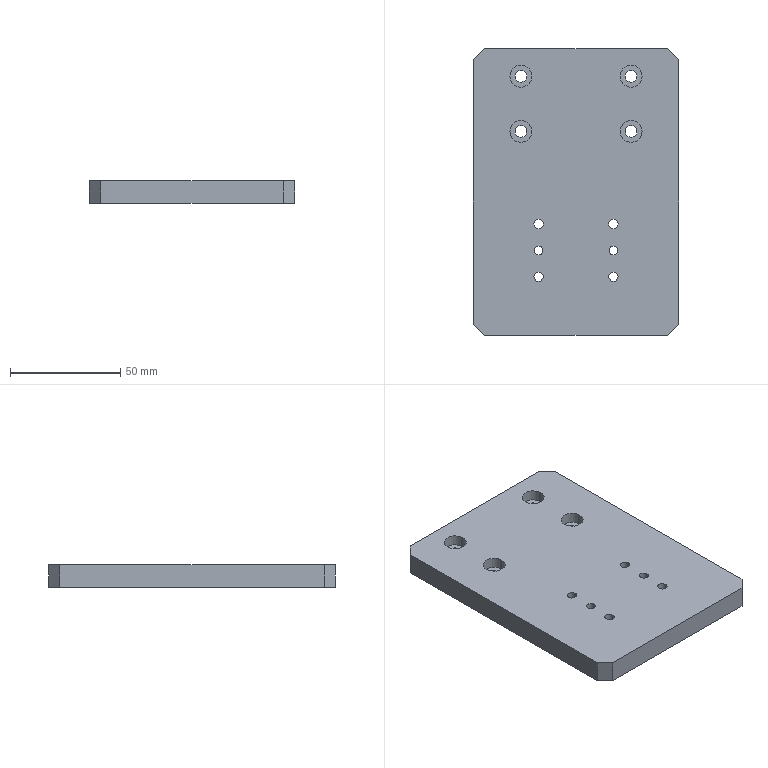Part | STEP file | CON-018 | 1 solid | 42 faces | box 93 x 130 x 10 mm | volume 117582 mm3 | cylinder 28 | plane 14 | commonest cylinder face diameters 4.2 x8 5.3 x8 10 x8 4 x4